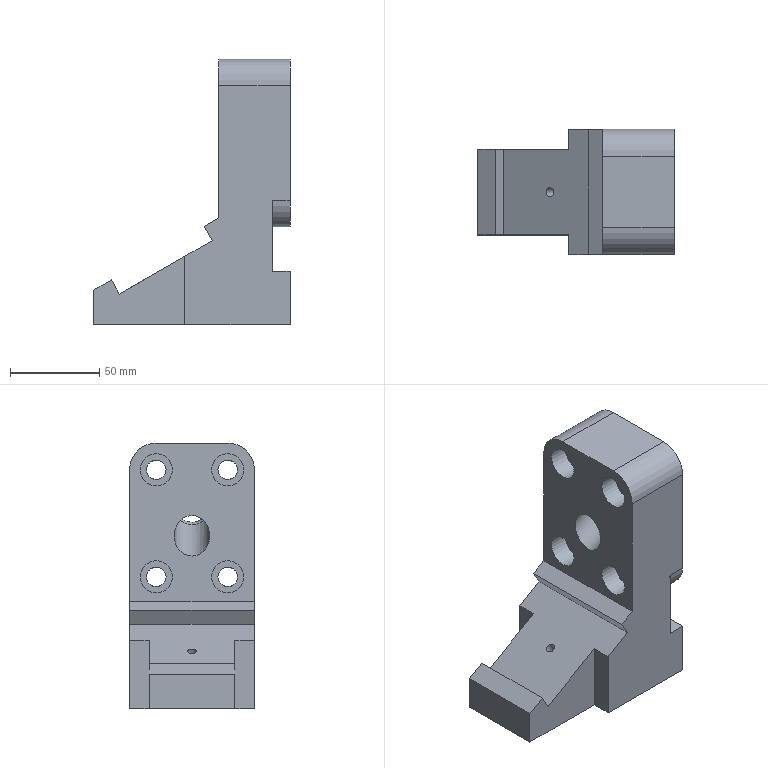Part | STEP file | solid 1 | 1 solid | 42 faces | box 110 x 70 x 149 mm | volume 483474 mm3 | plane 26 | cylinder 15 | cone 1 | commonest cylinder face diameters 11 x4 18 x4 30 x4 5 x1 20 x1 24 x1